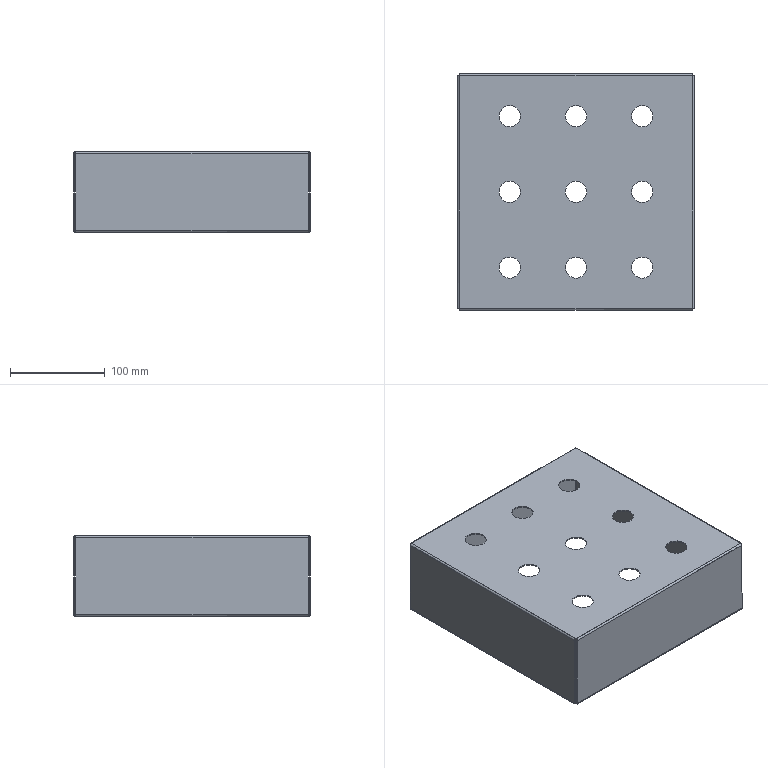Part | SolidWorks | features BaseBody 1 | 1 solid | 96 faces | box 250 x 250 x 85 mm | volume 198245 mm3 | cylinder 42 | plane 38 | spline 16 | commonest cylinder face diameters 22.5 x18 1.473 x8 3.873 x8 6.5 x8